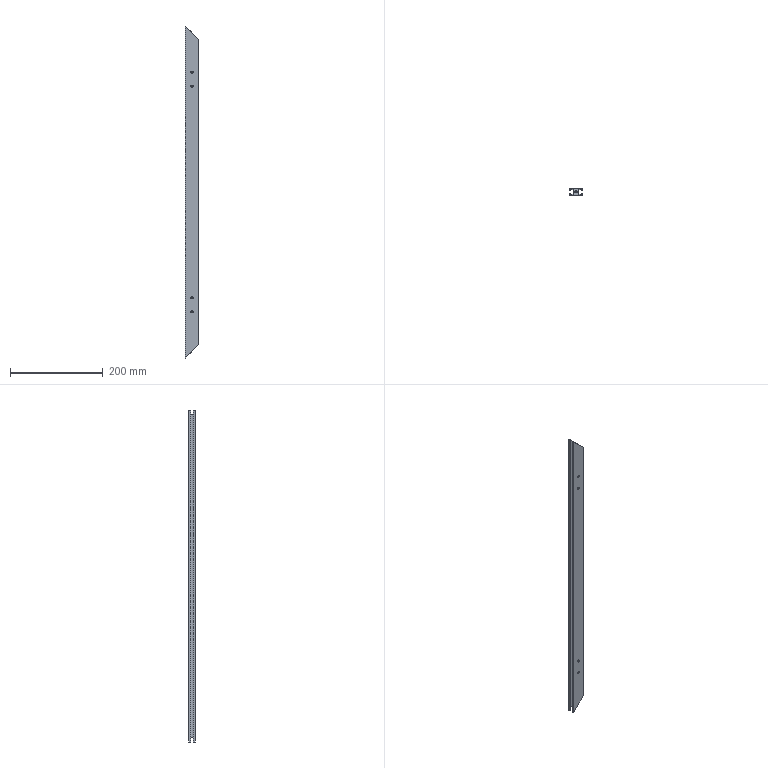Part | SolidWorks | features Extrusion 1, HoleWzd 1, ICE 1 | 1 solid | 49 faces | box 30 x 15 x 717 mm | volume 163021 mm3 | cylinder 29 | plane 20 | commonest cylinder face diameters 5 x26 16.345 x2 16.33 x1